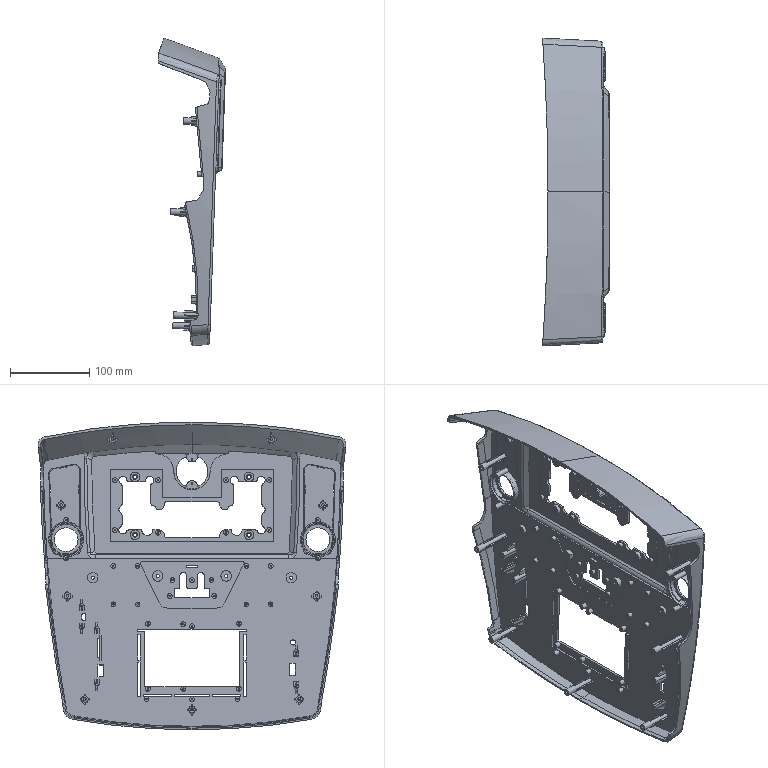Part | STEP file | MANIFOLD_SOLID_BREP_204099 | 1 solid | 1044 faces | box 84.491 x 387.927 x 387.413 mm | volume 502411 mm3 | plane 545 | cylinder 283 | spline 186 | cone 30 | commonest cylinder face diameters 6 x67 2 x41 10 x16 8 x13 2.5 x12 12 x11